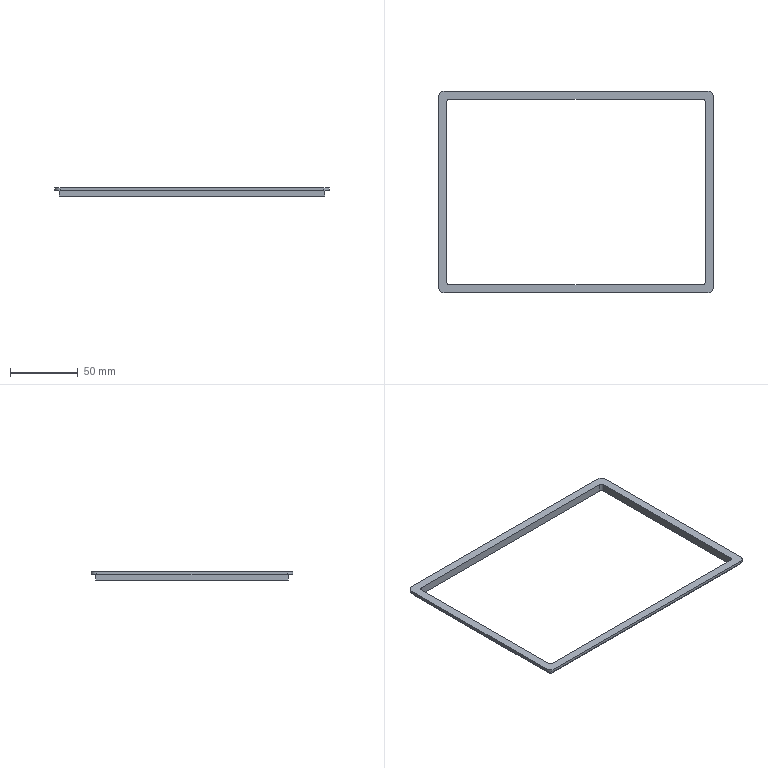Part | SolidWorks | features BaseBody 1 | 1 solid | 23 faces | box 203 x 149 x 6 mm | volume 14813 mm3 | plane 15 | cylinder 8 | commonest cylinder face diameters 4 x4 8 x4
STEP:
#1=CARTESIAN_POINT('',(-157.249,-26.46,0.));
#2=VERTEX_POINT('',#1);
#3=CARTESIAN_POINT('',(37.751,-26.46,0.));
#4=VERTEX_POINT('',#3);
#5=CARTESIAN_POINT('',(-161.249,-26.46,0.));
#6=DIRECTION('',(1.,0.,0.));
#7=VECTOR('',#6,1000.);
#8=LINE('',#5,#7);
#9=EDGE_CURVE('',#2,#4,#8,.T.);
#10=ORIENTED_EDGE('',*,*,#9,.F.);
#11=CARTESIAN_POINT('',(-161.249,-22.46,0.));
#12=VERTEX_POINT('',#11);
#13=CARTESIAN_POINT('',(-157.249,-22.46,0.));
#14=DIRECTION('',(0.,0.,-1.));
#15=DIRECTION('',(1.,0.,0.));
#16=AXIS2_PLACEMENT_3D('',#13,#14,#15);
#17=CIRCLE('',#16,4.);
#18=EDGE_CURVE('',#2,#12,#17,.T.);
#19=ORIENTED_EDGE('',*,*,#18,.T.);
#20=CARTESIAN_POINT('',(-161.249,118.54,0.));
#21=VERTEX_POINT('',#20);
#22=CARTESIAN_POINT('',(-161.249,122.54,0.));
#23=DIRECTION('',(0.,-1.,0.));
#24=VECTOR('',#23,1000.);
#25=LINE('',#22,#24);
#26=EDGE_CURVE('',#21,#12,#25,.T.);
#27=ORIENTED_EDGE('',*,*,#26,.F.);
#28=CARTESIAN_POINT('',(-157.249,122.54,0.));
#29=VERTEX_POINT('',#28);
#30=CARTESIAN_POINT('',(-157.249,118.54,0.));
#31=DIRECTION('',(0.,0.,-1.));
#32=DIRECTION('',(1.,0.,0.));
#33=AXIS2_PLACEMENT_3D('',#30,#31,#32);
#34=CIRCLE('',#33,4.);
#35=EDGE_CURVE('',#21,#29,#34,.T.);
#36=ORIENTED_EDGE('',*,*,#35,.T.);
#37=CARTESIAN_POINT('',(37.751,122.54,0.));
#38=VERTEX_POINT('',#37);
#39=CARTESIAN_POINT('',(41.751,122.54,0.));
#40=DIRECTION('',(-1.,0.,0.));
#41=VECTOR('',#40,1000.);
#42=LINE('',#39,#41);
#43=EDGE_CURVE('',#38,#29,#42,.T.);
#44=ORIENTED_EDGE('',*,*,#43,.F.);
#45=CARTESIAN_POINT('',(41.751,118.54,0.));
#46=VERTEX_POINT('',#45);
#47=CARTESIAN_POINT('',(37.751,118.54,0.));
#48=DIRECTION('',(0.,0.,-1.));
#49=DIRECTION('',(1.,0.,0.));
#50=AXIS2_PLACEMENT_3D('',#47,#48,#49);
#51=CIRCLE('',#50,4.);
#52=EDGE_CURVE('',#38,#46,#51,.T.);
#53=ORIENTED_EDGE('',*,*,#52,.T.);
#54=CARTESIAN_POINT('',(41.751,-22.46,0.));
#55=VERTEX_POINT('',#54);
#56=CARTESIAN_POINT('',(41.751,-26.46,0.));
#57=DIRECTION('',(0.,1.,0.));
#58=VECTOR('',#57,1000.);
#59=LINE('',#56,#58);
#60=EDGE_CURVE('',#55,#46,#59,.T.);
#61=ORIENTED_EDGE('',*,*,#60,.F.);
#62=CARTESIAN_POINT('',(37.751,-22.46,0.));
#63=DIRECTION('',(0.,0.,-1.));
#64=DIRECTION('',(1.,0.,0.));
#65=AXIS2_PLACEMENT_3D('',#62,#63,#64);
#66=CIRCLE('',#65,4.);
#67=EDGE_CURVE('',#55,#4,#66,.T.);
#68=ORIENTED_EDGE('',*,*,#67,.T.);
#69=EDGE_LOOP('',(#10,#19,#27,#36,#44,#53,#61,#68));
#70=FACE_OUTER_BOUND('',#69,.T.);
#71=CARTESIAN_POINT('',(-157.749,-22.96,0.));
#72=VERTEX_POINT('',#71);
#73=CARTESIAN_POINT('',(-157.749,119.04,0.));
#74=VERTEX_POINT('',#73);
#75=CARTESIAN_POINT('',(-157.749,119.04,0.));
#76=DIRECTION('',(0.,1.,0.));
#77=VECTOR('',#76,1000.);
#78=LINE('',#75,#77);
#79=EDGE_CURVE('',#72,#74,#78,.T.);
#80=ORIENTED_EDGE('',*,*,#79,.F.);
#81=CARTESIAN_POINT('',(38.251,-22.96,0.));
#82=VERTEX_POINT('',#81);
#83=CARTESIAN_POINT('',(-157.749,-22.96,0.));
#84=DIRECTION('',(-1.,0.,0.));
#85=VECTOR('',#84,1000.);
#86=LINE('',#83,#85);
#87=EDGE_CURVE('',#82,#72,#86,.T.);
#88=ORIENTED_EDGE('',*,*,#87,.F.);
#89=CARTESIAN_POINT('',(38.251,119.04,0.));
#90=VERTEX_POINT('',#89);
#91=CARTESIAN_POINT('',(38.251,-22.96,0.));
#92=DIRECTION('',(0.,-1.,0.));
#93=VECTOR('',#92,1000.);
#94=LINE('',#91,#93);
#95=EDGE_CURVE('',#90,#82,#94,.T.);
#96=ORIENTED_EDGE('',*,*,#95,.F.);
#97=CARTESIAN_POINT('',(38.251,119.04,0.));
#98=DIRECTION('',(1.,0.,0.));
#99=VECTOR('',#98,1000.);
#100=LINE('',#97,#99);
#101=EDGE_CURVE('',#74,#90,#100,.T.);
#102=ORIENTED_EDGE('',*,*,#101,.F.);
#103=EDGE_LOOP('',(#80,#88,#96,#102));
#104=FACE_BOUND('',#103,.T.);
#105=CARTESIAN_POINT('',(-161.249,-26.46,0.));
#106=DIRECTION('',(0.,0.,1.));
#107=DIRECTION('',(1.,0.,0.));
#108=AXIS2_PLACEMENT_3D('',#105,#106,#107);
#109=PLANE('',#108);
#110=ADVANCED_FACE('',(#70,#104),#109,.F.);
#111=CARTESIAN_POINT('',(-161.249,118.54,2.));
#112=VERTEX_POINT('',#111);
#113=CARTESIAN_POINT('',(-161.249,-22.46,2.));
#114=VERTEX_POINT('',#113);
#115=CARTESIAN_POINT('',(-161.249,122.54,2.));
#116=DIRECTION('',(0.,-1.,0.));
#117=VECTOR('',#116,1000.);
#118=LINE('',#115,#117);
#119=EDGE_CURVE('',#112,#114,#118,.T.);
#120=ORIENTED_EDGE('',*,*,#119,.T.);
#121=CARTESIAN_POINT('',(-157.249,-26.46,2.));
#122=VERTEX_POINT('',#121);
#123=CARTESIAN_POINT('',(-157.249,-22.46,2.));
#124=DIRECTION('',(0.,0.,1.));
#125=DIRECTION('',(1.,0.,0.));
#126=AXIS2_PLACEMENT_3D('',#123,#124,#125);
#127=CIRCLE('',#126,4.);
#128=EDGE_CURVE('',#114,#122,#127,.T.);
#129=ORIENTED_EDGE('',*,*,#128,.T.);
#130=CARTESIAN_POINT('',(37.751,-26.46,2.));
#131=VERTEX_POINT('',#130);
#132=CARTESIAN_POINT('',(-161.249,-26.46,2.));
#133=DIRECTION('',(1.,0.,0.));
#134=VECTOR('',#133,1000.);
#135=LINE('',#132,#134);
#136=EDGE_CURVE('',#122,#131,#135,.T.);
#137=ORIENTED_EDGE('',*,*,#136,.T.);
#138=CARTESIAN_POINT('',(41.751,-22.46,2.));
#139=VERTEX_POINT('',#138);
#140=CARTESIAN_POINT('',(37.751,-22.46,2.));
#141=DIRECTION('',(0.,0.,1.));
#142=DIRECTION('',(1.,0.,0.));
#143=AXIS2_PLACEMENT_3D('',#140,#141,#142);
#144=CIRCLE('',#143,4.);
#145=EDGE_CURVE('',#131,#139,#144,.T.);
#146=ORIENTED_EDGE('',*,*,#145,.T.);
#147=CARTESIAN_POINT('',(41.751,118.54,2.));
#148=VERTEX_POINT('',#147);
#149=CARTESIAN_POINT('',(41.751,-26.46,2.));
#150=DIRECTION('',(0.,1.,0.));
#151=VECTOR('',#150,1000.);
#152=LINE('',#149,#151);
#153=EDGE_CURVE('',#139,#148,#152,.T.);
#154=ORIENTED_EDGE('',*,*,#153,.T.);
#155=CARTESIAN_POINT('',(37.751,122.54,2.));
#156=VERTEX_POINT('',#155);
#157=CARTESIAN_POINT('',(37.751,118.54,2.));
#158=DIRECTION('',(0.,0.,1.));
#159=DIRECTION('',(1.,0.,0.));
#160=AXIS2_PLACEMENT_3D('',#157,#158,#159);
#161=CIRCLE('',#160,4.);
#162=EDGE_CURVE('',#148,#156,#161,.T.);
#163=ORIENTED_EDGE('',*,*,#162,.T.);
#164=CARTESIAN_POINT('',(-157.249,122.54,2.));
#165=VERTEX_POINT('',#164);
#166=CARTESIAN_POINT('',(41.751,122.54,2.));
#167=DIRECTION('',(-1.,0.,0.));
#168=VECTOR('',#167,1000.);
#169=LINE('',#166,#168);
#170=EDGE_CURVE('',#156,#165,#169,.T.);
#171=ORIENTED_EDGE('',*,*,#170,.T.);
#172=CARTESIAN_POINT('',(-157.249,118.54,2.));
#173=DIRECTION('',(0.,0.,1.));
#174=DIRECTION('',(1.,0.,0.));
#175=AXIS2_PLACEMENT_3D('',#172,#173,#174);
#176=CIRCLE('',#175,4.);
#177=EDGE_CURVE('',#165,#112,#176,.T.);
#178=ORIENTED_EDGE('',*,*,#177,.T.);
#179=EDGE_LOOP('',(#120,#129,#137,#146,#154,#163,#171,#178));
#180=FACE_OUTER_BOUND('',#179,.T.);
#181=CARTESIAN_POINT('',(-155.249,114.54,2.));
#182=VERTEX_POINT('',#181);
#183=CARTESIAN_POINT('',(-155.249,-18.46,2.));
#184=VERTEX_POINT('',#183);
#185=CARTESIAN_POINT('',(-155.249,116.54,2.));
#186=DIRECTION('',(0.,-1.,0.));
#187=VECTOR('',#186,1000.);
#188=LINE('',#185,#187);
#189=EDGE_CURVE('',#182,#184,#188,.T.);
#190=ORIENTED_EDGE('',*,*,#189,.F.);
#191=CARTESIAN_POINT('',(-153.249,116.54,2.));
#192=VERTEX_POINT('',#191);
#193=CARTESIAN_POINT('',(-153.249,114.54,2.));
#194=DIRECTION('',(0.,0.,-1.));
#195=DIRECTION('',(1.,0.,0.));
#196=AXIS2_PLACEMENT_3D('',#193,#194,#195);
#197=CIRCLE('',#196,2.);
#198=EDGE_CURVE('',#182,#192,#197,.T.);
#199=ORIENTED_EDGE('',*,*,#198,.T.);
#200=CARTESIAN_POINT('',(33.751,116.54,2.));
#201=VERTEX_POINT('',#200);
#202=CARTESIAN_POINT('',(35.751,116.54,2.));
#203=DIRECTION('',(-1.,0.,0.));
#204=VECTOR('',#203,1000.);
#205=LINE('',#202,#204);
#206=EDGE_CURVE('',#201,#192,#205,.T.);
#207=ORIENTED_EDGE('',*,*,#206,.F.);
#208=CARTESIAN_POINT('',(35.751,114.54,2.));
#209=VERTEX_POINT('',#208);
#210=CARTESIAN_POINT('',(33.751,114.54,2.));
#211=DIRECTION('',(0.,0.,-1.));
#212=DIRECTION('',(1.,0.,0.));
#213=AXIS2_PLACEMENT_3D('',#210,#211,#212);
#214=CIRCLE('',#213,2.);
#215=EDGE_CURVE('',#201,#209,#214,.T.);
#216=ORIENTED_EDGE('',*,*,#215,.T.);
#217=CARTESIAN_POINT('',(35.751,-18.46,2.));
#218=VERTEX_POINT('',#217);
#219=CARTESIAN_POINT('',(35.751,-20.46,2.));
#220=DIRECTION('',(0.,1.,0.));
#221=VECTOR('',#220,1000.);
#222=LINE('',#219,#221);
#223=EDGE_CURVE('',#218,#209,#222,.T.);
#224=ORIENTED_EDGE('',*,*,#223,.F.);
#225=CARTESIAN_POINT('',(33.751,-20.46,2.));
#226=VERTEX_POINT('',#225);
#227=CARTESIAN_POINT('',(33.751,-18.46,2.));
#228=DIRECTION('',(0.,0.,-1.));
#229=DIRECTION('',(1.,0.,0.));
#230=AXIS2_PLACEMENT_3D('',#227,#228,#229);
#231=CIRCLE('',#230,2.);
#232=EDGE_CURVE('',#218,#226,#231,.T.);
#233=ORIENTED_EDGE('',*,*,#232,.T.);
#234=CARTESIAN_POINT('',(-153.249,-20.46,2.));
#235=VERTEX_POINT('',#234);
#236=CARTESIAN_POINT('',(-155.249,-20.46,2.));
#237=DIRECTION('',(1.,0.,0.));
#238=VECTOR('',#237,1000.);
#239=LINE('',#236,#238);
#240=EDGE_CURVE('',#235,#226,#239,.T.);
#241=ORIENTED_EDGE('',*,*,#240,.F.);
#242=CARTESIAN_POINT('',(-153.249,-18.46,2.));
#243=DIRECTION('',(0.,0.,-1.));
#244=DIRECTION('',(1.,0.,0.));
#245=AXIS2_PLACEMENT_3D('',#242,#243,#244);
#246=CIRCLE('',#245,2.);
#247=EDGE_CURVE('',#235,#184,#246,.T.);
#248=ORIENTED_EDGE('',*,*,#247,.T.);
#249=EDGE_LOOP('',(#190,#199,#207,#216,#224,#233,#241,#248));
#250=FACE_BOUND('',#249,.T.);
#251=CARTESIAN_POINT('',(-161.249,-26.46,2.));
#252=DIRECTION('',(0.,0.,1.));
#253=DIRECTION('',(1.,0.,0.));
#254=AXIS2_PLACEMENT_3D('',#251,#252,#253);
#255=PLANE('',#254);
#256=ADVANCED_FACE('',(#180,#250),#255,.T.);
#257=ORIENTED_EDGE('',*,*,#26,.T.);
#258=CARTESIAN_POINT('',(-161.249,-22.46,2.));
#259=DIRECTION('',(0.,0.,1.));
#260=VECTOR('',#259,1000.);
#261=LINE('',#258,#260);
#262=EDGE_CURVE('',#12,#114,#261,.T.);
#263=ORIENTED_EDGE('',*,*,#262,.T.);
#264=ORIENTED_EDGE('',*,*,#119,.F.);
#265=CARTESIAN_POINT('',(-161.249,118.54,2.));
#266=DIRECTION('',(0.,0.,-1.));
#267=VECTOR('',#266,1000.);
#268=LINE('',#265,#267);
#269=EDGE_CURVE('',#112,#21,#268,.T.);
#270=ORIENTED_EDGE('',*,*,#269,.T.);
#271=EDGE_LOOP('',(#257,#263,#264,#270));
#272=FACE_OUTER_BOUND('',#271,.T.);
#273=CARTESIAN_POINT('',(-161.249,122.54,2.));
#274=DIRECTION('',(1.,0.,0.));
#275=DIRECTION('',(0.,0.,-1.));
#276=AXIS2_PLACEMENT_3D('',#273,#274,#275);
#277=PLANE('',#276);
#278=ADVANCED_FACE('',(#272),#277,.F.);
#279=ORIENTED_EDGE('',*,*,#136,.F.);
#280=CARTESIAN_POINT('',(-157.249,-26.46,2.));
#281=DIRECTION('',(0.,0.,-1.));
#282=VECTOR('',#281,1000.);
#283=LINE('',#280,#282);
#284=EDGE_CURVE('',#122,#2,#283,.T.);
#285=ORIENTED_EDGE('',*,*,#284,.T.);
#286=ORIENTED_EDGE('',*,*,#9,.T.);
#287=CARTESIAN_POINT('',(37.751,-26.46,2.));
#288=DIRECTION('',(0.,0.,1.));
#289=VECTOR('',#288,1000.);
#290=LINE('',#287,#289);
#291=EDGE_CURVE('',#4,#131,#290,.T.);
#292=ORIENTED_EDGE('',*,*,#291,.T.);
#293=EDGE_LOOP('',(#279,#285,#286,#292));
#294=FACE_OUTER_BOUND('',#293,.T.);
#295=CARTESIAN_POINT('',(-161.249,-26.46,2.));
#296=DIRECTION('',(0.,1.,0.));
#297=DIRECTION('',(0.,0.,1.));
#298=AXIS2_PLACEMENT_3D('',#295,#296,#297);
#299=PLANE('',#298);
#300=ADVANCED_FACE('',(#294),#299,.F.);
#301=ORIENTED_EDGE('',*,*,#60,.T.);
#302=CARTESIAN_POINT('',(41.751,118.54,2.));
#303=DIRECTION('',(0.,0.,1.));
#304=VECTOR('',#303,1000.);
#305=LINE('',#302,#304);
#306=EDGE_CURVE('',#46,#148,#305,.T.);
#307=ORIENTED_EDGE('',*,*,#306,.T.);
#308=ORIENTED_EDGE('',*,*,#153,.F.);
#309=CARTESIAN_POINT('',(41.751,-22.46,2.));
#310=DIRECTION('',(0.,0.,-1.));
#311=VECTOR('',#310,1000.);
#312=LINE('',#309,#311);
#313=EDGE_CURVE('',#139,#55,#312,.T.);
#314=ORIENTED_EDGE('',*,*,#313,.T.);
#315=EDGE_LOOP('',(#301,#307,#308,#314));
#316=FACE_OUTER_BOUND('',#315,.T.);
#317=CARTESIAN_POINT('',(41.751,-26.46,2.));
#318=DIRECTION('',(-1.,0.,0.));
#319=DIRECTION('',(0.,0.,1.));
#320=AXIS2_PLACEMENT_3D('',#317,#318,#319);
#321=PLANE('',#320);
#322=ADVANCED_FACE('',(#316),#321,.F.);
#323=ORIENTED_EDGE('',*,*,#43,.T.);
#324=CARTESIAN_POINT('',(-157.249,122.54,2.));
#325=DIRECTION('',(0.,0.,1.));
#326=VECTOR('',#325,1000.);
#327=LINE('',#324,#326);
#328=EDGE_CURVE('',#29,#165,#327,.T.);
#329=ORIENTED_EDGE('',*,*,#328,.T.);
#330=ORIENTED_EDGE('',*,*,#170,.F.);
#331=CARTESIAN_POINT('',(37.751,122.54,2.));
#332=DIRECTION('',(0.,0.,-1.));
#333=VECTOR('',#332,1000.);
#334=LINE('',#331,#333);
#335=EDGE_CURVE('',#156,#38,#334,.T.);
#336=ORIENTED_EDGE('',*,*,#335,.T.);
#337=EDGE_LOOP('',(#323,#329,#330,#336));
#338=FACE_OUTER_BOUND('',#337,.T.);
#339=CARTESIAN_POINT('',(41.751,122.54,2.));
#340=DIRECTION('',(0.,-1.,0.));
#341=DIRECTION('',(0.,0.,-1.));
#342=AXIS2_PLACEMENT_3D('',#339,#340,#341);
#343=PLANE('',#342);
#344=ADVANCED_FACE('',(#338),#343,.F.);
#345=CARTESIAN_POINT('',(-153.249,116.54,-4.));
#346=VERTEX_POINT('',#345);
#347=CARTESIAN_POINT('',(33.751,116.54,-4.));
#348=VERTEX_POINT('',#347);
#349=CARTESIAN_POINT('',(35.751,116.54,-4.));
#350=DIRECTION('',(1.,0.,0.));
#351=VECTOR('',#350,1000.);
#352=LINE('',#349,#351);
#353=EDGE_CURVE('',#346,#348,#352,.T.);
#354=ORIENTED_EDGE('',*,*,#353,.T.);
#355=CARTESIAN_POINT('',(33.751,116.54,2.));
#356=DIRECTION('',(0.,0.,1.));
#357=VECTOR('',#356,1000.);
#358=LINE('',#355,#357);
#359=EDGE_CURVE('',#348,#201,#358,.T.);
#360=ORIENTED_EDGE('',*,*,#359,.T.);
#361=ORIENTED_EDGE('',*,*,#206,.T.);
#362=CARTESIAN_POINT('',(-153.249,116.54,-4.));
#363=DIRECTION('',(0.,0.,-1.));
#364=VECTOR('',#363,1000.);
#365=LINE('',#362,#364);
#366=EDGE_CURVE('',#192,#346,#365,.T.);
#367=ORIENTED_EDGE('',*,*,#366,.T.);
#368=EDGE_LOOP('',(#354,#360,#361,#367));
#369=FACE_OUTER_BOUND('',#368,.T.);
#370=CARTESIAN_POINT('',(35.751,116.54,2.));
#371=DIRECTION('',(0.,-1.,0.));
#372=DIRECTION('',(0.,0.,-1.));
#373=AXIS2_PLACEMENT_3D('',#370,#371,#372);
#374=PLANE('',#373);
#375=ADVANCED_FACE('',(#369),#374,.T.);
#376=CARTESIAN_POINT('',(-155.249,-18.46,-4.));
#377=VERTEX_POINT('',#376);
#378=CARTESIAN_POINT('',(-155.249,114.54,-4.));
#379=VERTEX_POINT('',#378);
#380=CARTESIAN_POINT('',(-155.249,116.54,-4.));
#381=DIRECTION('',(0.,1.,0.));
#382=VECTOR('',#381,1000.);
#383=LINE('',#380,#382);
#384=EDGE_CURVE('',#377,#379,#383,.T.);
#385=ORIENTED_EDGE('',*,*,#384,.T.);
#386=CARTESIAN_POINT('',(-155.249,114.54,2.));
#387=DIRECTION('',(0.,0.,1.));
#388=VECTOR('',#387,1000.);
#389=LINE('',#386,#388);
#390=EDGE_CURVE('',#379,#182,#389,.T.);
#391=ORIENTED_EDGE('',*,*,#390,.T.);
#392=ORIENTED_EDGE('',*,*,#189,.T.);
#393=CARTESIAN_POINT('',(-155.249,-18.46,-4.));
#394=DIRECTION('',(0.,0.,-1.));
#395=VECTOR('',#394,1000.);
#396=LINE('',#393,#395);
#397=EDGE_CURVE('',#184,#377,#396,.T.);
#398=ORIENTED_EDGE('',*,*,#397,.T.);
#399=EDGE_LOOP('',(#385,#391,#392,#398));
#400=FACE_OUTER_BOUND('',#399,.T.);
#401=CARTESIAN_POINT('',(-155.249,116.54,2.));
#402=DIRECTION('',(1.,0.,0.));
#403=DIRECTION('',(0.,0.,-1.));
#404=AXIS2_PLACEMENT_3D('',#401,#402,#403);
#405=PLANE('',#404);
#406=ADVANCED_FACE('',(#400),#405,.T.);
#407=ORIENTED_EDGE('',*,*,#240,.T.);
#408=CARTESIAN_POINT('',(33.751,-20.46,-4.));
#409=VERTEX_POINT('',#408);
#410=CARTESIAN_POINT('',(33.751,-20.46,-4.));
#411=DIRECTION('',(0.,0.,-1.));
#412=VECTOR('',#411,1000.);
#413=LINE('',#410,#412);
#414=EDGE_CURVE('',#226,#409,#413,.T.);
#415=ORIENTED_EDGE('',*,*,#414,.T.);
#416=CARTESIAN_POINT('',(-153.249,-20.46,-4.));
#417=VERTEX_POINT('',#416);
#418=CARTESIAN_POINT('',(-155.249,-20.46,-4.));
#419=DIRECTION('',(-1.,0.,0.));
#420=VECTOR('',#419,1000.);
#421=LINE('',#418,#420);
#422=EDGE_CURVE('',#409,#417,#421,.T.);
#423=ORIENTED_EDGE('',*,*,#422,.T.);
#424=CARTESIAN_POINT('',(-153.249,-20.46,2.));
#425=DIRECTION('',(0.,0.,1.));
#426=VECTOR('',#425,1000.);
#427=LINE('',#424,#426);
#428=EDGE_CURVE('',#417,#235,#427,.T.);
#429=ORIENTED_EDGE('',*,*,#428,.T.);
#430=EDGE_LOOP('',(#407,#415,#423,#429));
#431=FACE_OUTER_BOUND('',#430,.T.);
#432=CARTESIAN_POINT('',(-155.249,-20.46,2.));
#433=DIRECTION('',(0.,1.,0.));
#434=DIRECTION('',(0.,0.,1.));
#435=AXIS2_PLACEMENT_3D('',#432,#433,#434);
#436=PLANE('',#435);
#437=ADVANCED_FACE('',(#431),#436,.T.);
#438=CARTESIAN_POINT('',(35.751,114.54,-4.));
#439=VERTEX_POINT('',#438);
#440=CARTESIAN_POINT('',(35.751,-18.46,-4.));
#441=VERTEX_POINT('',#440);
#442=CARTESIAN_POINT('',(35.751,-20.46,-4.));
#443=DIRECTION('',(0.,-1.,0.));
#444=VECTOR('',#443,1000.);
#445=LINE('',#442,#444);
#446=EDGE_CURVE('',#439,#441,#445,.T.);
#447=ORIENTED_EDGE('',*,*,#446,.T.);
#448=CARTESIAN_POINT('',(35.751,-18.46,2.));
#449=DIRECTION('',(0.,0.,1.));
#450=VECTOR('',#449,1000.);
#451=LINE('',#448,#450);
#452=EDGE_CURVE('',#441,#218,#451,.T.);
#453=ORIENTED_EDGE('',*,*,#452,.T.);
#454=ORIENTED_EDGE('',*,*,#223,.T.);
#455=CARTESIAN_POINT('',(35.751,114.54,-4.));
#456=DIRECTION('',(0.,0.,-1.));
#457=VECTOR('',#456,1000.);
#458=LINE('',#455,#457);
#459=EDGE_CURVE('',#209,#439,#458,.T.);
#460=ORIENTED_EDGE('',*,*,#459,.T.);
#461=EDGE_LOOP('',(#447,#453,#454,#460));
#462=FACE_OUTER_BOUND('',#461,.T.);
#463=CARTESIAN_POINT('',(35.751,-20.46,2.));
#464=DIRECTION('',(-1.,0.,0.));
#465=DIRECTION('',(0.,0.,1.));
#466=AXIS2_PLACEMENT_3D('',#463,#464,#465);
#467=PLANE('',#466);
#468=ADVANCED_FACE('',(#462),#467,.T.);
#469=CARTESIAN_POINT('',(-157.749,-22.96,-4.));
#470=VERTEX_POINT('',#469);
#471=CARTESIAN_POINT('',(-157.749,119.04,-4.));
#472=VERTEX_POINT('',#471);
#473=CARTESIAN_POINT('',(-157.749,119.04,-4.));
#474=DIRECTION('',(0.,1.,0.));
#475=VECTOR('',#474,1000.);
#476=LINE('',#473,#475);
#477=EDGE_CURVE('',#470,#472,#476,.T.);
#478=ORIENTED_EDGE('',*,*,#477,.T.);
#479=CARTESIAN_POINT('',(38.251,119.04,-4.));
#480=VERTEX_POINT('',#479);
#481=CARTESIAN_POINT('',(38.251,119.04,-4.));
#482=DIRECTION('',(1.,0.,0.));
#483=VECTOR('',#482,1000.);
#484=LINE('',#481,#483);
#485=EDGE_CURVE('',#472,#480,#484,.T.);
#486=ORIENTED_EDGE('',*,*,#485,.T.);
#487=CARTESIAN_POINT('',(38.251,-22.96,-4.));
#488=VERTEX_POINT('',#487);
#489=CARTESIAN_POINT('',(38.251,-22.96,-4.));
#490=DIRECTION('',(0.,-1.,0.));
#491=VECTOR('',#490,1000.);
#492=LINE('',#489,#491);
#493=EDGE_CURVE('',#480,#488,#492,.T.);
#494=ORIENTED_EDGE('',*,*,#493,.T.);
#495=CARTESIAN_POINT('',(-157.749,-22.96,-4.));
#496=DIRECTION('',(-1.,0.,0.));
#497=VECTOR('',#496,1000.);
#498=LINE('',#495,#497);
#499=EDGE_CURVE('',#488,#470,#498,.T.);
#500=ORIENTED_EDGE('',*,*,#499,.T.);
#501=EDGE_LOOP('',(#478,#486,#494,#500));
#502=FACE_OUTER_BOUND('',#501,.T.);
#503=ORIENTED_EDGE('',*,*,#422,.F.);
#504=CARTESIAN_POINT('',(33.751,-18.46,-4.));
#505=DIRECTION('',(0.,0.,1.));
#506=DIRECTION('',(1.,0.,0.));
#507=AXIS2_PLACEMENT_3D('',#504,#505,#506);
#508=CIRCLE('',#507,2.);
#509=EDGE_CURVE('',#409,#441,#508,.T.);
#510=ORIENTED_EDGE('',*,*,#509,.T.);
#511=ORIENTED_EDGE('',*,*,#446,.F.);
#512=CARTESIAN_POINT('',(33.751,114.54,-4.));
#513=DIRECTION('',(0.,0.,1.));
#514=DIRECTION('',(1.,0.,0.));
#515=AXIS2_PLACEMENT_3D('',#512,#513,#514);
#516=CIRCLE('',#515,2.);
#517=EDGE_CURVE('',#439,#348,#516,.T.);
#518=ORIENTED_EDGE('',*,*,#517,.T.);
#519=ORIENTED_EDGE('',*,*,#353,.F.);
#520=CARTESIAN_POINT('',(-153.249,114.54,-4.));
#521=DIRECTION('',(0.,0.,1.));
#522=DIRECTION('',(1.,0.,0.));
#523=AXIS2_PLACEMENT_3D('',#520,#521,#522);
#524=CIRCLE('',#523,2.);
#525=EDGE_CURVE('',#346,#379,#524,.T.);
#526=ORIENTED_EDGE('',*,*,#525,.T.);
#527=ORIENTED_EDGE('',*,*,#384,.F.);
#528=CARTESIAN_POINT('',(-153.249,-18.46,-4.));
#529=DIRECTION('',(0.,0.,1.));
#530=DIRECTION('',(1.,0.,0.));
#531=AXIS2_PLACEMENT_3D('',#528,#529,#530);
#532=CIRCLE('',#531,2.);
#533=EDGE_CURVE('',#377,#417,#532,.T.);
#534=ORIENTED_EDGE('',*,*,#533,.T.);
#535=EDGE_LOOP('',(#503,#510,#511,#518,#519,#526,#527,#534));
#536=FACE_BOUND('',#535,.T.);
#537=CARTESIAN_POINT('',(-157.749,-22.96,-4.));
#538=DIRECTION('',(0.,0.,1.));
#539=DIRECTION('',(1.,0.,0.));
#540=AXIS2_PLACEMENT_3D('',#537,#538,#539);
#541=PLANE('',#540);
#542=ADVANCED_FACE('',(#502,#536),#541,.F.);
#543=ORIENTED_EDGE('',*,*,#79,.T.);
#544=CARTESIAN_POINT('',(-157.749,119.04,-4.));
#545=DIRECTION('',(0.,0.,1.));
#546=VECTOR('',#545,1000.);
#547=LINE('',#544,#546);
#548=EDGE_CURVE('',#472,#74,#547,.T.);
#549=ORIENTED_EDGE('',*,*,#548,.F.);
#550=ORIENTED_EDGE('',*,*,#477,.F.);
#551=CARTESIAN_POINT('',(-157.749,-22.96,-4.));
#552=DIRECTION('',(0.,0.,1.));
#553=VECTOR('',#552,1000.);
#554=LINE('',#551,#553);
#555=EDGE_CURVE('',#470,#72,#554,.T.);
#556=ORIENTED_EDGE('',*,*,#555,.T.);
#557=EDGE_LOOP('',(#543,#549,#550,#556));
#558=FACE_OUTER_BOUND('',#557,.T.);
#559=CARTESIAN_POINT('',(-157.749,119.04,-4.));
#560=DIRECTION('',(1.,0.,0.));
#561=DIRECTION('',(0.,0.,-1.));
#562=AXIS2_PLACEMENT_3D('',#559,#560,#561);
#563=PLANE('',#562);
#564=ADVANCED_FACE('',(#558),#563,.F.);
#565=ORIENTED_EDGE('',*,*,#101,.T.);
#566=CARTESIAN_POINT('',(38.251,119.04,-4.));
#567=DIRECTION('',(0.,0.,1.));
#568=VECTOR('',#567,1000.);
#569=LINE('',#566,#568);
#570=EDGE_CURVE('',#480,#90,#569,.T.);
#571=ORIENTED_EDGE('',*,*,#570,.F.);
#572=ORIENTED_EDGE('',*,*,#485,.F.);
#573=ORIENTED_EDGE('',*,*,#548,.T.);
#574=EDGE_LOOP('',(#565,#571,#572,#573));
#575=FACE_OUTER_BOUND('',#574,.T.);
#576=CARTESIAN_POINT('',(38.251,119.04,-4.));
#577=DIRECTION('',(0.,-1.,0.));
#578=DIRECTION('',(0.,0.,-1.));
#579=AXIS2_PLACEMENT_3D('',#576,#577,#578);
#580=PLANE('',#579);
#581=ADVANCED_FACE('',(#575),#580,.F.);
#582=ORIENTED_EDGE('',*,*,#95,.T.);
#583=CARTESIAN_POINT('',(38.251,-22.96,-4.));
#584=DIRECTION('',(0.,0.,1.));
#585=VECTOR('',#584,1000.);
#586=LINE('',#583,#585);
#587=EDGE_CURVE('',#488,#82,#586,.T.);
#588=ORIENTED_EDGE('',*,*,#587,.F.);
#589=ORIENTED_EDGE('',*,*,#493,.F.);
#590=ORIENTED_EDGE('',*,*,#570,.T.);
#591=EDGE_LOOP('',(#582,#588,#589,#590));
#592=FACE_OUTER_BOUND('',#591,.T.);
#593=CARTESIAN_POINT('',(38.251,-22.96,-4.));
#594=DIRECTION('',(-1.,0.,0.));
#595=DIRECTION('',(0.,0.,1.));
#596=AXIS2_PLACEMENT_3D('',#593,#594,#595);
#597=PLANE('',#596);
#598=ADVANCED_FACE('',(#592),#597,.F.);
#599=ORIENTED_EDGE('',*,*,#87,.T.);
#600=ORIENTED_EDGE('',*,*,#555,.F.);
#601=ORIENTED_EDGE('',*,*,#499,.F.);
#602=ORIENTED_EDGE('',*,*,#587,.T.);
#603=EDGE_LOOP('',(#599,#600,#601,#602));
#604=FACE_OUTER_BOUND('',#603,.T.);
#605=CARTESIAN_POINT('',(-157.749,-22.96,-4.));
#606=DIRECTION('',(0.,1.,0.));
#607=DIRECTION('',(0.,0.,1.));
#608=AXIS2_PLACEMENT_3D('',#605,#606,#607);
#609=PLANE('',#608);
#610=ADVANCED_FACE('',(#604),#609,.F.);
#611=ORIENTED_EDGE('',*,*,#128,.F.);
#612=ORIENTED_EDGE('',*,*,#262,.F.);
#613=ORIENTED_EDGE('',*,*,#18,.F.);
#614=ORIENTED_EDGE('',*,*,#284,.F.);
#615=EDGE_LOOP('',(#611,#612,#613,#614));
#616=FACE_OUTER_BOUND('',#615,.T.);
#617=CARTESIAN_POINT('',(-157.249,-22.46,2.));
#618=DIRECTION('',(0.,0.,-1.));
#619=DIRECTION('',(-1.,0.,0.));
#620=AXIS2_PLACEMENT_3D('',#617,#618,#619);
#621=CYLINDRICAL_SURFACE('',#620,4.);
#622=ADVANCED_FACE('',(#616),#621,.T.);
#623=ORIENTED_EDGE('',*,*,#177,.F.);
#624=ORIENTED_EDGE('',*,*,#328,.F.);
#625=ORIENTED_EDGE('',*,*,#35,.F.);
#626=ORIENTED_EDGE('',*,*,#269,.F.);
#627=EDGE_LOOP('',(#623,#624,#625,#626));
#628=FACE_OUTER_BOUND('',#627,.T.);
#629=CARTESIAN_POINT('',(-157.249,118.54,2.));
#630=DIRECTION('',(0.,0.,-1.));
#631=DIRECTION('',(-1.,0.,0.));
#632=AXIS2_PLACEMENT_3D('',#629,#630,#631);
#633=CYLINDRICAL_SURFACE('',#632,4.);
#634=ADVANCED_FACE('',(#628),#633,.T.);
#635=ORIENTED_EDGE('',*,*,#162,.F.);
#636=ORIENTED_EDGE('',*,*,#306,.F.);
#637=ORIENTED_EDGE('',*,*,#52,.F.);
#638=ORIENTED_EDGE('',*,*,#335,.F.);
#639=EDGE_LOOP('',(#635,#636,#637,#638));
#640=FACE_OUTER_BOUND('',#639,.T.);
#641=CARTESIAN_POINT('',(37.751,118.54,2.));
#642=DIRECTION('',(0.,0.,-1.));
#643=DIRECTION('',(-1.,0.,0.));
#644=AXIS2_PLACEMENT_3D('',#641,#642,#643);
#645=CYLINDRICAL_SURFACE('',#644,4.);
#646=ADVANCED_FACE('',(#640),#645,.T.);
#647=ORIENTED_EDGE('',*,*,#145,.F.);
#648=ORIENTED_EDGE('',*,*,#291,.F.);
#649=ORIENTED_EDGE('',*,*,#67,.F.);
#650=ORIENTED_EDGE('',*,*,#313,.F.);
#651=EDGE_LOOP('',(#647,#648,#649,#650));
#652=FACE_OUTER_BOUND('',#651,.T.);
#653=CARTESIAN_POINT('',(37.751,-22.46,2.));
#654=DIRECTION('',(0.,0.,-1.));
#655=DIRECTION('',(-1.,0.,0.));
#656=AXIS2_PLACEMENT_3D('',#653,#654,#655);
#657=CYLINDRICAL_SURFACE('',#656,4.);
#658=ADVANCED_FACE('',(#652),#657,.T.);
#659=ORIENTED_EDGE('',*,*,#232,.F.);
#660=ORIENTED_EDGE('',*,*,#452,.F.);
#661=ORIENTED_EDGE('',*,*,#509,.F.);
#662=ORIENTED_EDGE('',*,*,#414,.F.);
#663=EDGE_LOOP('',(#659,#660,#661,#662));
#664=FACE_OUTER_BOUND('',#663,.T.);
#665=CARTESIAN_POINT('',(33.751,-18.46,2.));
#666=DIRECTION('',(0.,0.,1.));
#667=DIRECTION('',(1.,0.,0.));
#668=AXIS2_PLACEMENT_3D('',#665,#666,#667);
#669=CYLINDRICAL_SURFACE('',#668,2.);
#670=ADVANCED_FACE('',(#664),#669,.F.);
#671=ORIENTED_EDGE('',*,*,#215,.F.);
#672=ORIENTED_EDGE('',*,*,#359,.F.);
#673=ORIENTED_EDGE('',*,*,#517,.F.);
#674=ORIENTED_EDGE('',*,*,#459,.F.);
#675=EDGE_LOOP('',(#671,#672,#673,#674));
#676=FACE_OUTER_BOUND('',#675,.T.);
#677=CARTESIAN_POINT('',(33.751,114.54,2.));
#678=DIRECTION('',(0.,0.,1.));
#679=DIRECTION('',(1.,0.,0.));
#680=AXIS2_PLACEMENT_3D('',#677,#678,#679);
#681=CYLINDRICAL_SURFACE('',#680,2.);
#682=ADVANCED_FACE('',(#676),#681,.F.);
#683=ORIENTED_EDGE('',*,*,#198,.F.);
#684=ORIENTED_EDGE('',*,*,#390,.F.);
#685=ORIENTED_EDGE('',*,*,#525,.F.);
#686=ORIENTED_EDGE('',*,*,#366,.F.);
#687=EDGE_LOOP('',(#683,#684,#685,#686));
#688=FACE_OUTER_BOUND('',#687,.T.);
#689=CARTESIAN_POINT('',(-153.249,114.54,2.));
#690=DIRECTION('',(0.,0.,1.));
#691=DIRECTION('',(1.,0.,0.));
#692=AXIS2_PLACEMENT_3D('',#689,#690,#691);
#693=CYLINDRICAL_SURFACE('',#692,2.);
#694=ADVANCED_FACE('',(#688),#693,.F.);
#695=ORIENTED_EDGE('',*,*,#247,.F.);
#696=ORIENTED_EDGE('',*,*,#428,.F.);
#697=ORIENTED_EDGE('',*,*,#533,.F.);
#698=ORIENTED_EDGE('',*,*,#397,.F.);
#699=EDGE_LOOP('',(#695,#696,#697,#698));
#700=FACE_OUTER_BOUND('',#699,.T.);
#701=CARTESIAN_POINT('',(-153.249,-18.46,2.));
#702=DIRECTION('',(0.,0.,1.));
#703=DIRECTION('',(1.,0.,0.));
#704=AXIS2_PLACEMENT_3D('',#701,#702,#703);
#705=CYLINDRICAL_SURFACE('',#704,2.);
#706=ADVANCED_FACE('',(#700),#705,.F.);
#707=CLOSED_SHELL('',(#110,#256,#278,#300,#322,#344,#375,#406,#437,#468,#542,#564,#581,#598,#610,#622,#634,#646,#658,#670,#682,#694,#706));
#708=MANIFOLD_SOLID_BREP('',#707);
#709=CARTESIAN_POINT('',(0.,0.,0.));
#710=DIRECTION('',(0.,0.,1.));
#711=DIRECTION('',(1.,0.,0.));
#712=AXIS2_PLACEMENT_3D('',#709,#710,#711);
#713=(LENGTH_UNIT()NAMED_UNIT(*)SI_UNIT(.MILLI.,.METRE.));
#714=UNCERTAINTY_MEASURE_WITH_UNIT(LENGTH_MEASURE(0.00001),#713,'','');
#715=(NAMED_UNIT(*)PLANE_ANGLE_UNIT()SI_UNIT($,.RADIAN.));
#716=(NAMED_UNIT(*)SI_UNIT($,.STERADIAN.)SOLID_ANGLE_UNIT());
#717=(GEOMETRIC_REPRESENTATION_CONTEXT(3)GLOBAL_UNCERTAINTY_ASSIGNED_CONTEXT((#714))GLOBAL_UNIT_ASSIGNED_CONTEXT((#713,#715,#716))REPRESENTATION_CONTEXT('',''));
#718=ADVANCED_BREP_SHAPE_REPRESENTATION('',(#708,#712),#717);